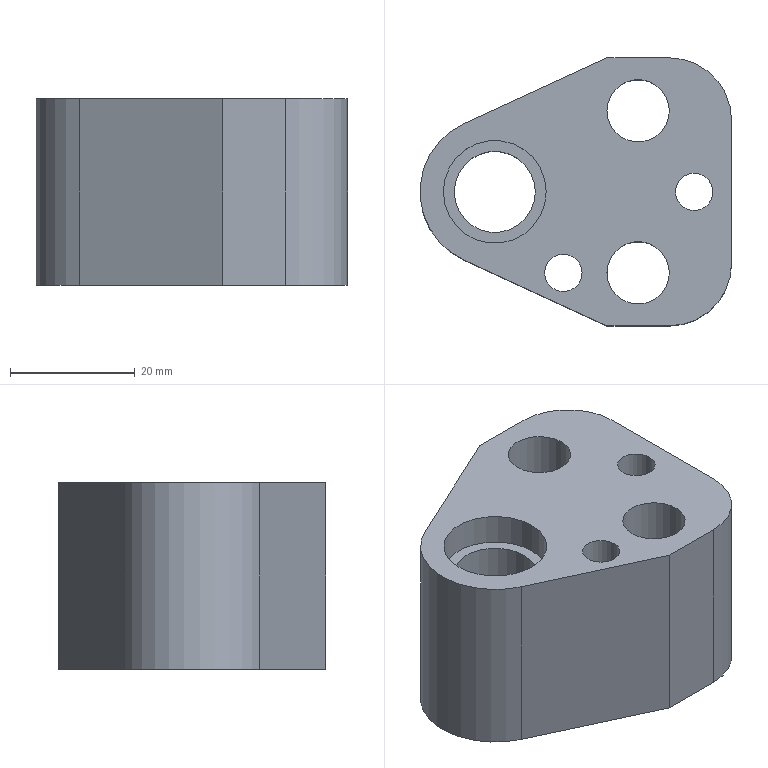Part | NX | features solid 2 | 1 solid | 25 faces | box 50 x 43 x 30 mm | volume 36983 mm3 | cylinder 13 | plane 12 | commonest cylinder face diameters 6 x2 8 x2 10 x2 14 x2 20 x2 13 x1
STEP:
#1=CARTESIAN_POINT('',(1616.,131.992,72.));
#2=VERTEX_POINT('',#1);
#3=CARTESIAN_POINT('',(1620.,131.992,72.));
#4=DIRECTION('',(0.,0.,-1.));
#5=DIRECTION('',(-1.,0.,0.));
#6=AXIS2_PLACEMENT_3D('',#3,#4,#5);
#7=CIRCLE('',#6,4.);
#8=EDGE_CURVE('',#2,#2,#7,.F.);
#9=ORIENTED_EDGE('',*,*,#8,.T.);
#10=EDGE_LOOP('',(#9));
#11=FACE_BOUND('',#10,.T.);
#12=CARTESIAN_POINT('',(1618.,118.992,72.));
#13=VERTEX_POINT('',#12);
#14=CARTESIAN_POINT('',(1611.,118.992,72.));
#15=DIRECTION('',(0.,0.,1.));
#16=DIRECTION('',(1.,0.,0.));
#17=AXIS2_PLACEMENT_3D('',#14,#15,#16);
#18=CIRCLE('',#17,7.);
#19=EDGE_CURVE('',#13,#13,#18,.T.);
#20=ORIENTED_EDGE('',*,*,#19,.T.);
#21=EDGE_LOOP('',(#20));
#22=FACE_BOUND('',#21,.T.);
#23=CARTESIAN_POINT('',(1618.,144.992,72.));
#24=VERTEX_POINT('',#23);
#25=CARTESIAN_POINT('',(1611.,144.992,72.));
#26=DIRECTION('',(0.,0.,1.));
#27=DIRECTION('',(1.,0.,0.));
#28=AXIS2_PLACEMENT_3D('',#25,#26,#27);
#29=CIRCLE('',#28,7.);
#30=EDGE_CURVE('',#24,#24,#29,.T.);
#31=ORIENTED_EDGE('',*,*,#30,.T.);
#32=EDGE_LOOP('',(#31));
#33=FACE_BOUND('',#32,.T.);
#34=CARTESIAN_POINT('',(1581.5,131.992,72.));
#35=VERTEX_POINT('',#34);
#36=CARTESIAN_POINT('',(1588.,131.992,72.));
#37=DIRECTION('',(0.,0.,-1.));
#38=DIRECTION('',(-1.,0.,0.));
#39=AXIS2_PLACEMENT_3D('',#36,#37,#38);
#40=CIRCLE('',#39,6.5);
#41=EDGE_CURVE('',#35,#35,#40,.T.);
#42=ORIENTED_EDGE('',*,*,#41,.F.);
#43=EDGE_LOOP('',(#42));
#44=FACE_BOUND('',#43,.T.);
#45=CARTESIAN_POINT('',(1582.981,142.892,72.));
#46=VERTEX_POINT('',#45);
#47=CARTESIAN_POINT('',(1606.,153.492,72.));
#48=VERTEX_POINT('',#47);
#49=CARTESIAN_POINT('',(1582.981,142.892,72.));
#50=DIRECTION('',(0.9083,0.4183,0.));
#51=VECTOR('',#50,1000.);
#52=LINE('',#49,#51);
#53=EDGE_CURVE('',#46,#48,#52,.T.);
#54=ORIENTED_EDGE('',*,*,#53,.T.);
#55=CARTESIAN_POINT('',(1616.,153.492,72.));
#56=VERTEX_POINT('',#55);
#57=CARTESIAN_POINT('',(1606.,153.492,72.));
#58=DIRECTION('',(1.,0.,0.));
#59=VECTOR('',#58,1000.);
#60=LINE('',#57,#59);
#61=EDGE_CURVE('',#48,#56,#60,.T.);
#62=ORIENTED_EDGE('',*,*,#61,.T.);
#63=CARTESIAN_POINT('',(1626.,143.492,72.));
#64=VERTEX_POINT('',#63);
#65=CARTESIAN_POINT('',(1616.,143.492,72.));
#66=DIRECTION('',(0.,0.,1.));
#67=DIRECTION('',(1.,0.,0.));
#68=AXIS2_PLACEMENT_3D('',#65,#66,#67);
#69=CIRCLE('',#68,10.);
#70=EDGE_CURVE('',#64,#56,#69,.T.);
#71=ORIENTED_EDGE('',*,*,#70,.F.);
#72=CARTESIAN_POINT('',(1626.,120.492,72.));
#73=VERTEX_POINT('',#72);
#74=CARTESIAN_POINT('',(1626.,143.492,72.));
#75=DIRECTION('',(0.,-1.,0.));
#76=VECTOR('',#75,1000.);
#77=LINE('',#74,#76);
#78=EDGE_CURVE('',#64,#73,#77,.T.);
#79=ORIENTED_EDGE('',*,*,#78,.T.);
#80=CARTESIAN_POINT('',(1616.,110.492,72.));
#81=VERTEX_POINT('',#80);
#82=CARTESIAN_POINT('',(1616.,120.492,72.));
#83=DIRECTION('',(0.,0.,1.));
#84=DIRECTION('',(1.,0.,0.));
#85=AXIS2_PLACEMENT_3D('',#82,#83,#84);
#86=CIRCLE('',#85,10.);
#87=EDGE_CURVE('',#81,#73,#86,.T.);
#88=ORIENTED_EDGE('',*,*,#87,.F.);
#89=CARTESIAN_POINT('',(1606.,110.492,72.));
#90=VERTEX_POINT('',#89);
#91=CARTESIAN_POINT('',(1606.,110.492,72.));
#92=DIRECTION('',(1.,0.,0.));
#93=VECTOR('',#92,1000.);
#94=LINE('',#91,#93);
#95=EDGE_CURVE('',#90,#81,#94,.T.);
#96=ORIENTED_EDGE('',*,*,#95,.F.);
#97=CARTESIAN_POINT('',(1582.981,121.093,72.));
#98=VERTEX_POINT('',#97);
#99=CARTESIAN_POINT('',(1582.981,121.093,72.));
#100=DIRECTION('',(0.9083,-0.4183,0.));
#101=VECTOR('',#100,1000.);
#102=LINE('',#99,#101);
#103=EDGE_CURVE('',#98,#90,#102,.T.);
#104=ORIENTED_EDGE('',*,*,#103,.F.);
#105=CARTESIAN_POINT('',(1588.,131.992,72.));
#106=DIRECTION('',(0.,0.,1.));
#107=DIRECTION('',(1.,0.,0.));
#108=AXIS2_PLACEMENT_3D('',#105,#106,#107);
#109=CIRCLE('',#108,12.);
#110=EDGE_CURVE('',#46,#98,#109,.T.);
#111=ORIENTED_EDGE('',*,*,#110,.F.);
#112=EDGE_LOOP('',(#54,#62,#71,#79,#88,#96,#104,#111));
#113=FACE_BOUND('',#112,.T.);
#114=CARTESIAN_POINT('',(1595.,118.992,72.));
#115=VERTEX_POINT('',#114);
#116=CARTESIAN_POINT('',(1599.,118.992,72.));
#117=DIRECTION('',(0.,0.,-1.));
#118=DIRECTION('',(-1.,0.,0.));
#119=AXIS2_PLACEMENT_3D('',#116,#117,#118);
#120=CIRCLE('',#119,4.);
#121=EDGE_CURVE('',#115,#115,#120,.F.);
#122=ORIENTED_EDGE('',*,*,#121,.T.);
#123=EDGE_LOOP('',(#122));
#124=FACE_BOUND('',#123,.T.);
#125=CARTESIAN_POINT('',(1616.,143.492,72.));
#126=DIRECTION('',(0.,0.,-1.));
#127=DIRECTION('',(1.,0.,0.));
#128=AXIS2_PLACEMENT_3D('',#125,#126,#127);
#129=PLANE('',#128);
#130=ADVANCED_FACE('',(#11,#22,#33,#44,#113,#124),#129,.T.);
#131=CARTESIAN_POINT('',(1623.,131.992,102.));
#132=VERTEX_POINT('',#131);
#133=CARTESIAN_POINT('',(1620.,131.992,102.));
#134=DIRECTION('',(0.,0.,1.));
#135=DIRECTION('',(1.,0.,0.));
#136=AXIS2_PLACEMENT_3D('',#133,#134,#135);
#137=CIRCLE('',#136,3.);
#138=EDGE_CURVE('',#132,#132,#137,.T.);
#139=ORIENTED_EDGE('',*,*,#138,.T.);
#140=EDGE_LOOP('',(#139));
#141=FACE_BOUND('',#140,.T.);
#142=CARTESIAN_POINT('',(1623.,131.992,92.));
#143=VERTEX_POINT('',#142);
#144=CARTESIAN_POINT('',(1620.,131.992,92.));
#145=DIRECTION('',(0.,0.,1.));
#146=DIRECTION('',(1.,0.,0.));
#147=AXIS2_PLACEMENT_3D('',#144,#145,#146);
#148=CIRCLE('',#147,3.);
#149=EDGE_CURVE('',#143,#143,#148,.T.);
#150=ORIENTED_EDGE('',*,*,#149,.F.);
#151=EDGE_LOOP('',(#150));
#152=FACE_BOUND('',#151,.T.);
#153=CARTESIAN_POINT('',(1620.,131.992,72.));
#154=DIRECTION('',(0.,0.,1.));
#155=DIRECTION('',(-1.,0.,0.));
#156=AXIS2_PLACEMENT_3D('',#153,#154,#155);
#157=CYLINDRICAL_SURFACE('',#156,3.);
#158=ADVANCED_FACE('',(#141,#152),#157,.F.);
#159=CARTESIAN_POINT('',(1616.,118.992,102.));
#160=VERTEX_POINT('',#159);
#161=CARTESIAN_POINT('',(1611.,118.992,102.));
#162=DIRECTION('',(0.,0.,1.));
#163=DIRECTION('',(1.,0.,0.));
#164=AXIS2_PLACEMENT_3D('',#161,#162,#163);
#165=CIRCLE('',#164,5.);
#166=EDGE_CURVE('',#160,#160,#165,.T.);
#167=ORIENTED_EDGE('',*,*,#166,.T.);
#168=EDGE_LOOP('',(#167));
#169=FACE_BOUND('',#168,.T.);
#170=CARTESIAN_POINT('',(1616.,118.992,82.));
#171=VERTEX_POINT('',#170);
#172=CARTESIAN_POINT('',(1611.,118.992,82.));
#173=DIRECTION('',(0.,0.,1.));
#174=DIRECTION('',(1.,0.,0.));
#175=AXIS2_PLACEMENT_3D('',#172,#173,#174);
#176=CIRCLE('',#175,5.);
#177=EDGE_CURVE('',#171,#171,#176,.T.);
#178=ORIENTED_EDGE('',*,*,#177,.F.);
#179=EDGE_LOOP('',(#178));
#180=FACE_BOUND('',#179,.T.);
#181=CARTESIAN_POINT('',(1611.,118.992,72.));
#182=DIRECTION('',(0.,0.,1.));
#183=DIRECTION('',(-1.,0.,0.));
#184=AXIS2_PLACEMENT_3D('',#181,#182,#183);
#185=CYLINDRICAL_SURFACE('',#184,5.);
#186=ADVANCED_FACE('',(#169,#180),#185,.F.);
#187=CARTESIAN_POINT('',(1616.,144.992,102.));
#188=VERTEX_POINT('',#187);
#189=CARTESIAN_POINT('',(1611.,144.992,102.));
#190=DIRECTION('',(0.,0.,1.));
#191=DIRECTION('',(1.,0.,0.));
#192=AXIS2_PLACEMENT_3D('',#189,#190,#191);
#193=CIRCLE('',#192,5.);
#194=EDGE_CURVE('',#188,#188,#193,.T.);
#195=ORIENTED_EDGE('',*,*,#194,.T.);
#196=EDGE_LOOP('',(#195));
#197=FACE_BOUND('',#196,.T.);
#198=CARTESIAN_POINT('',(1616.,144.992,82.));
#199=VERTEX_POINT('',#198);
#200=CARTESIAN_POINT('',(1611.,144.992,82.));
#201=DIRECTION('',(0.,0.,1.));
#202=DIRECTION('',(1.,0.,0.));
#203=AXIS2_PLACEMENT_3D('',#200,#201,#202);
#204=CIRCLE('',#203,5.);
#205=EDGE_CURVE('',#199,#199,#204,.T.);
#206=ORIENTED_EDGE('',*,*,#205,.F.);
#207=EDGE_LOOP('',(#206));
#208=FACE_BOUND('',#207,.T.);
#209=CARTESIAN_POINT('',(1611.,144.992,72.));
#210=DIRECTION('',(0.,0.,1.));
#211=DIRECTION('',(-1.,0.,0.));
#212=AXIS2_PLACEMENT_3D('',#209,#210,#211);
#213=CYLINDRICAL_SURFACE('',#212,5.);
#214=ADVANCED_FACE('',(#197,#208),#213,.F.);
#215=CARTESIAN_POINT('',(1602.,118.992,102.));
#216=VERTEX_POINT('',#215);
#217=CARTESIAN_POINT('',(1599.,118.992,102.));
#218=DIRECTION('',(0.,0.,1.));
#219=DIRECTION('',(1.,0.,0.));
#220=AXIS2_PLACEMENT_3D('',#217,#218,#219);
#221=CIRCLE('',#220,3.);
#222=EDGE_CURVE('',#216,#216,#221,.T.);
#223=ORIENTED_EDGE('',*,*,#222,.F.);
#224=EDGE_LOOP('',(#223));
#225=FACE_BOUND('',#224,.T.);
#226=ORIENTED_EDGE('',*,*,#166,.F.);
#227=EDGE_LOOP('',(#226));
#228=FACE_BOUND('',#227,.T.);
#229=CARTESIAN_POINT('',(1582.981,142.892,102.));
#230=VERTEX_POINT('',#229);
#231=CARTESIAN_POINT('',(1606.,153.492,102.));
#232=VERTEX_POINT('',#231);
#233=CARTESIAN_POINT('',(1582.981,142.892,102.));
#234=DIRECTION('',(0.9083,0.4183,0.));
#235=VECTOR('',#234,1000.);
#236=LINE('',#233,#235);
#237=EDGE_CURVE('',#230,#232,#236,.T.);
#238=ORIENTED_EDGE('',*,*,#237,.F.);
#239=CARTESIAN_POINT('',(1582.981,121.093,102.));
#240=VERTEX_POINT('',#239);
#241=CARTESIAN_POINT('',(1588.,131.992,102.));
#242=DIRECTION('',(0.,0.,1.));
#243=DIRECTION('',(1.,0.,0.));
#244=AXIS2_PLACEMENT_3D('',#241,#242,#243);
#245=CIRCLE('',#244,12.);
#246=EDGE_CURVE('',#230,#240,#245,.T.);
#247=ORIENTED_EDGE('',*,*,#246,.T.);
#248=CARTESIAN_POINT('',(1606.,110.492,102.));
#249=VERTEX_POINT('',#248);
#250=CARTESIAN_POINT('',(1582.981,121.093,102.));
#251=DIRECTION('',(0.9083,-0.4183,0.));
#252=VECTOR('',#251,1000.);
#253=LINE('',#250,#252);
#254=EDGE_CURVE('',#240,#249,#253,.T.);
#255=ORIENTED_EDGE('',*,*,#254,.T.);
#256=CARTESIAN_POINT('',(1616.,110.492,102.));
#257=VERTEX_POINT('',#256);
#258=CARTESIAN_POINT('',(1606.,110.492,102.));
#259=DIRECTION('',(1.,0.,0.));
#260=VECTOR('',#259,1000.);
#261=LINE('',#258,#260);
#262=EDGE_CURVE('',#249,#257,#261,.T.);
#263=ORIENTED_EDGE('',*,*,#262,.T.);
#264=CARTESIAN_POINT('',(1626.,120.492,102.));
#265=VERTEX_POINT('',#264);
#266=CARTESIAN_POINT('',(1616.,120.492,102.));
#267=DIRECTION('',(0.,0.,1.));
#268=DIRECTION('',(1.,0.,0.));
#269=AXIS2_PLACEMENT_3D('',#266,#267,#268);
#270=CIRCLE('',#269,10.);
#271=EDGE_CURVE('',#257,#265,#270,.T.);
#272=ORIENTED_EDGE('',*,*,#271,.T.);
#273=CARTESIAN_POINT('',(1626.,143.492,102.));
#274=VERTEX_POINT('',#273);
#275=CARTESIAN_POINT('',(1626.,143.492,102.));
#276=DIRECTION('',(0.,-1.,0.));
#277=VECTOR('',#276,1000.);
#278=LINE('',#275,#277);
#279=EDGE_CURVE('',#274,#265,#278,.T.);
#280=ORIENTED_EDGE('',*,*,#279,.F.);
#281=CARTESIAN_POINT('',(1616.,153.492,102.));
#282=VERTEX_POINT('',#281);
#283=CARTESIAN_POINT('',(1616.,143.492,102.));
#284=DIRECTION('',(0.,0.,1.));
#285=DIRECTION('',(1.,0.,0.));
#286=AXIS2_PLACEMENT_3D('',#283,#284,#285);
#287=CIRCLE('',#286,10.);
#288=EDGE_CURVE('',#274,#282,#287,.T.);
#289=ORIENTED_EDGE('',*,*,#288,.T.);
#290=CARTESIAN_POINT('',(1606.,153.492,102.));
#291=DIRECTION('',(1.,0.,0.));
#292=VECTOR('',#291,1000.);
#293=LINE('',#290,#292);
#294=EDGE_CURVE('',#232,#282,#293,.T.);
#295=ORIENTED_EDGE('',*,*,#294,.F.);
#296=EDGE_LOOP('',(#238,#247,#255,#263,#272,#280,#289,#295));
#297=FACE_BOUND('',#296,.T.);
#298=CARTESIAN_POINT('',(1596.25,131.992,102.));
#299=VERTEX_POINT('',#298);
#300=CARTESIAN_POINT('',(1588.,131.992,102.));
#301=DIRECTION('',(0.,0.,1.));
#302=DIRECTION('',(1.,0.,0.));
#303=AXIS2_PLACEMENT_3D('',#300,#301,#302);
#304=CIRCLE('',#303,8.25);
#305=EDGE_CURVE('',#299,#299,#304,.T.);
#306=ORIENTED_EDGE('',*,*,#305,.F.);
#307=EDGE_LOOP('',(#306));
#308=FACE_BOUND('',#307,.T.);
#309=ORIENTED_EDGE('',*,*,#194,.F.);
#310=EDGE_LOOP('',(#309));
#311=FACE_BOUND('',#310,.T.);
#312=ORIENTED_EDGE('',*,*,#138,.F.);
#313=EDGE_LOOP('',(#312));
#314=FACE_BOUND('',#313,.T.);
#315=CARTESIAN_POINT('',(1616.,143.492,102.));
#316=DIRECTION('',(0.,0.,-1.));
#317=DIRECTION('',(1.,0.,0.));
#318=AXIS2_PLACEMENT_3D('',#315,#316,#317);
#319=PLANE('',#318);
#320=ADVANCED_FACE('',(#225,#228,#297,#308,#311,#314),#319,.F.);
#321=ORIENTED_EDGE('',*,*,#237,.T.);
#322=CARTESIAN_POINT('',(1606.,153.492,72.));
#323=DIRECTION('',(0.,0.,1.));
#324=VECTOR('',#323,1000.);
#325=LINE('',#322,#324);
#326=EDGE_CURVE('',#48,#232,#325,.T.);
#327=ORIENTED_EDGE('',*,*,#326,.F.);
#328=ORIENTED_EDGE('',*,*,#53,.F.);
#329=CARTESIAN_POINT('',(1582.981,142.892,72.));
#330=DIRECTION('',(0.,0.,1.));
#331=VECTOR('',#330,1000.);
#332=LINE('',#329,#331);
#333=EDGE_CURVE('',#46,#230,#332,.T.);
#334=ORIENTED_EDGE('',*,*,#333,.T.);
#335=EDGE_LOOP('',(#321,#327,#328,#334));
#336=FACE_BOUND('',#335,.T.);
#337=CARTESIAN_POINT('',(1582.981,142.892,72.));
#338=DIRECTION('',(-0.4183,0.9083,0.));
#339=DIRECTION('',(0.9083,0.4183,0.));
#340=AXIS2_PLACEMENT_3D('',#337,#338,#339);
#341=PLANE('',#340);
#342=ADVANCED_FACE('',(#336),#341,.T.);
#343=ORIENTED_EDGE('',*,*,#294,.T.);
#344=CARTESIAN_POINT('',(1616.,153.492,72.));
#345=DIRECTION('',(0.,0.,1.));
#346=VECTOR('',#345,1000.);
#347=LINE('',#344,#346);
#348=EDGE_CURVE('',#56,#282,#347,.T.);
#349=ORIENTED_EDGE('',*,*,#348,.F.);
#350=ORIENTED_EDGE('',*,*,#61,.F.);
#351=ORIENTED_EDGE('',*,*,#326,.T.);
#352=EDGE_LOOP('',(#343,#349,#350,#351));
#353=FACE_BOUND('',#352,.T.);
#354=CARTESIAN_POINT('',(1606.,153.492,72.));
#355=DIRECTION('',(0.,1.,0.));
#356=DIRECTION('',(1.,0.,0.));
#357=AXIS2_PLACEMENT_3D('',#354,#355,#356);
#358=PLANE('',#357);
#359=ADVANCED_FACE('',(#353),#358,.T.);
#360=ORIENTED_EDGE('',*,*,#288,.F.);
#361=CARTESIAN_POINT('',(1626.,143.492,72.));
#362=DIRECTION('',(0.,0.,1.));
#363=VECTOR('',#362,1000.);
#364=LINE('',#361,#363);
#365=EDGE_CURVE('',#64,#274,#364,.T.);
#366=ORIENTED_EDGE('',*,*,#365,.F.);
#367=ORIENTED_EDGE('',*,*,#70,.T.);
#368=ORIENTED_EDGE('',*,*,#348,.T.);
#369=EDGE_LOOP('',(#360,#366,#367,#368));
#370=FACE_BOUND('',#369,.T.);
#371=CARTESIAN_POINT('',(1616.,143.492,72.));
#372=DIRECTION('',(0.,0.,1.));
#373=DIRECTION('',(-1.,0.,0.));
#374=AXIS2_PLACEMENT_3D('',#371,#372,#373);
#375=CYLINDRICAL_SURFACE('',#374,10.);
#376=ADVANCED_FACE('',(#370),#375,.T.);
#377=ORIENTED_EDGE('',*,*,#279,.T.);
#378=CARTESIAN_POINT('',(1626.,120.492,72.));
#379=DIRECTION('',(0.,0.,1.));
#380=VECTOR('',#379,1000.);
#381=LINE('',#378,#380);
#382=EDGE_CURVE('',#73,#265,#381,.T.);
#383=ORIENTED_EDGE('',*,*,#382,.F.);
#384=ORIENTED_EDGE('',*,*,#78,.F.);
#385=ORIENTED_EDGE('',*,*,#365,.T.);
#386=EDGE_LOOP('',(#377,#383,#384,#385));
#387=FACE_BOUND('',#386,.T.);
#388=CARTESIAN_POINT('',(1626.,143.492,72.));
#389=DIRECTION('',(1.,0.,0.));
#390=DIRECTION('',(0.,-1.,0.));
#391=AXIS2_PLACEMENT_3D('',#388,#389,#390);
#392=PLANE('',#391);
#393=ADVANCED_FACE('',(#387),#392,.T.);
#394=ORIENTED_EDGE('',*,*,#271,.F.);
#395=CARTESIAN_POINT('',(1616.,110.492,72.));
#396=DIRECTION('',(0.,0.,1.));
#397=VECTOR('',#396,1000.);
#398=LINE('',#395,#397);
#399=EDGE_CURVE('',#81,#257,#398,.T.);
#400=ORIENTED_EDGE('',*,*,#399,.F.);
#401=ORIENTED_EDGE('',*,*,#87,.T.);
#402=ORIENTED_EDGE('',*,*,#382,.T.);
#403=EDGE_LOOP('',(#394,#400,#401,#402));
#404=FACE_BOUND('',#403,.T.);
#405=CARTESIAN_POINT('',(1616.,120.492,72.));
#406=DIRECTION('',(0.,0.,1.));
#407=DIRECTION('',(-1.,0.,0.));
#408=AXIS2_PLACEMENT_3D('',#405,#406,#407);
#409=CYLINDRICAL_SURFACE('',#408,10.);
#410=ADVANCED_FACE('',(#404),#409,.T.);
#411=ORIENTED_EDGE('',*,*,#262,.F.);
#412=CARTESIAN_POINT('',(1606.,110.492,72.));
#413=DIRECTION('',(0.,0.,1.));
#414=VECTOR('',#413,1000.);
#415=LINE('',#412,#414);
#416=EDGE_CURVE('',#90,#249,#415,.T.);
#417=ORIENTED_EDGE('',*,*,#416,.F.);
#418=ORIENTED_EDGE('',*,*,#95,.T.);
#419=ORIENTED_EDGE('',*,*,#399,.T.);
#420=EDGE_LOOP('',(#411,#417,#418,#419));
#421=FACE_BOUND('',#420,.T.);
#422=CARTESIAN_POINT('',(1606.,110.492,72.));
#423=DIRECTION('',(0.,1.,0.));
#424=DIRECTION('',(1.,0.,0.));
#425=AXIS2_PLACEMENT_3D('',#422,#423,#424);
#426=PLANE('',#425);
#427=ADVANCED_FACE('',(#421),#426,.F.);
#428=ORIENTED_EDGE('',*,*,#254,.F.);
#429=CARTESIAN_POINT('',(1582.981,121.093,72.));
#430=DIRECTION('',(0.,0.,1.));
#431=VECTOR('',#430,1000.);
#432=LINE('',#429,#431);
#433=EDGE_CURVE('',#98,#240,#432,.T.);
#434=ORIENTED_EDGE('',*,*,#433,.F.);
#435=ORIENTED_EDGE('',*,*,#103,.T.);
#436=ORIENTED_EDGE('',*,*,#416,.T.);
#437=EDGE_LOOP('',(#428,#434,#435,#436));
#438=FACE_BOUND('',#437,.T.);
#439=CARTESIAN_POINT('',(1582.981,121.093,72.));
#440=DIRECTION('',(0.4183,0.9083,0.));
#441=DIRECTION('',(0.9083,-0.4183,0.));
#442=AXIS2_PLACEMENT_3D('',#439,#440,#441);
#443=PLANE('',#442);
#444=ADVANCED_FACE('',(#438),#443,.F.);
#445=ORIENTED_EDGE('',*,*,#246,.F.);
#446=ORIENTED_EDGE('',*,*,#333,.F.);
#447=ORIENTED_EDGE('',*,*,#110,.T.);
#448=ORIENTED_EDGE('',*,*,#433,.T.);
#449=EDGE_LOOP('',(#445,#446,#447,#448));
#450=FACE_BOUND('',#449,.T.);
#451=CARTESIAN_POINT('',(1588.,131.992,72.));
#452=DIRECTION('',(0.,0.,1.));
#453=DIRECTION('',(-1.,0.,0.));
#454=AXIS2_PLACEMENT_3D('',#451,#452,#453);
#455=CYLINDRICAL_SURFACE('',#454,12.);
#456=ADVANCED_FACE('',(#450),#455,.T.);
#457=CARTESIAN_POINT('',(1594.5,131.992,97.));
#458=VERTEX_POINT('',#457);
#459=CARTESIAN_POINT('',(1588.,131.992,97.));
#460=DIRECTION('',(0.,0.,1.));
#461=DIRECTION('',(1.,0.,0.));
#462=AXIS2_PLACEMENT_3D('',#459,#460,#461);
#463=CIRCLE('',#462,6.5);
#464=EDGE_CURVE('',#458,#458,#463,.F.);
#465=ORIENTED_EDGE('',*,*,#464,.F.);
#466=EDGE_LOOP('',(#465));
#467=FACE_BOUND('',#466,.T.);
#468=ORIENTED_EDGE('',*,*,#41,.T.);
#469=EDGE_LOOP('',(#468));
#470=FACE_BOUND('',#469,.T.);
#471=CARTESIAN_POINT('',(1588.,131.992,72.));
#472=DIRECTION('',(0.,0.,1.));
#473=DIRECTION('',(-1.,0.,0.));
#474=AXIS2_PLACEMENT_3D('',#471,#472,#473);
#475=CYLINDRICAL_SURFACE('',#474,6.5);
#476=ADVANCED_FACE('',(#467,#470),#475,.F.);
#477=CARTESIAN_POINT('',(1596.25,131.992,97.));
#478=VERTEX_POINT('',#477);
#479=CARTESIAN_POINT('',(1588.,131.992,97.));
#480=DIRECTION('',(0.,0.,1.));
#481=DIRECTION('',(1.,0.,0.));
#482=AXIS2_PLACEMENT_3D('',#479,#480,#481);
#483=CIRCLE('',#482,8.25);
#484=EDGE_CURVE('',#478,#478,#483,.T.);
#485=ORIENTED_EDGE('',*,*,#484,.T.);
#486=EDGE_LOOP('',(#485));
#487=FACE_BOUND('',#486,.T.);
#488=ORIENTED_EDGE('',*,*,#464,.T.);
#489=EDGE_LOOP('',(#488));
#490=FACE_BOUND('',#489,.T.);
#491=CARTESIAN_POINT('',(1588.,131.992,97.));
#492=DIRECTION('',(0.,0.,-1.));
#493=DIRECTION('',(1.,0.,0.));
#494=AXIS2_PLACEMENT_3D('',#491,#492,#493);
#495=PLANE('',#494);
#496=ADVANCED_FACE('',(#487,#490),#495,.F.);
#497=ORIENTED_EDGE('',*,*,#484,.F.);
#498=EDGE_LOOP('',(#497));
#499=FACE_BOUND('',#498,.T.);
#500=ORIENTED_EDGE('',*,*,#305,.T.);
#501=EDGE_LOOP('',(#500));
#502=FACE_BOUND('',#501,.T.);
#503=CARTESIAN_POINT('',(1588.,131.992,97.));
#504=DIRECTION('',(0.,0.,1.));
#505=DIRECTION('',(-1.,0.,0.));
#506=AXIS2_PLACEMENT_3D('',#503,#504,#505);
#507=CYLINDRICAL_SURFACE('',#506,8.25);
#508=ADVANCED_FACE('',(#499,#502),#507,.F.);
#509=CARTESIAN_POINT('',(1602.,118.992,92.));
#510=VERTEX_POINT('',#509);
#511=CARTESIAN_POINT('',(1599.,118.992,92.));
#512=DIRECTION('',(0.,0.,1.));
#513=DIRECTION('',(1.,0.,0.));
#514=AXIS2_PLACEMENT_3D('',#511,#512,#513);
#515=CIRCLE('',#514,3.);
#516=EDGE_CURVE('',#510,#510,#515,.T.);
#517=ORIENTED_EDGE('',*,*,#516,.F.);
#518=EDGE_LOOP('',(#517));
#519=FACE_BOUND('',#518,.T.);
#520=ORIENTED_EDGE('',*,*,#222,.T.);
#521=EDGE_LOOP('',(#520));
#522=FACE_BOUND('',#521,.T.);
#523=CARTESIAN_POINT('',(1599.,118.992,72.));
#524=DIRECTION('',(0.,0.,1.));
#525=DIRECTION('',(-1.,0.,0.));
#526=AXIS2_PLACEMENT_3D('',#523,#524,#525);
#527=CYLINDRICAL_SURFACE('',#526,3.);
#528=ADVANCED_FACE('',(#519,#522),#527,.F.);
#529=CARTESIAN_POINT('',(1618.,144.992,82.));
#530=VERTEX_POINT('',#529);
#531=CARTESIAN_POINT('',(1611.,144.992,82.));
#532=DIRECTION('',(0.,0.,1.));
#533=DIRECTION('',(1.,0.,0.));
#534=AXIS2_PLACEMENT_3D('',#531,#532,#533);
#535=CIRCLE('',#534,7.);
#536=EDGE_CURVE('',#530,#530,#535,.T.);
#537=ORIENTED_EDGE('',*,*,#536,.T.);
#538=EDGE_LOOP('',(#537));
#539=FACE_BOUND('',#538,.T.);
#540=ORIENTED_EDGE('',*,*,#30,.F.);
#541=EDGE_LOOP('',(#540));
#542=FACE_BOUND('',#541,.T.);
#543=CARTESIAN_POINT('',(1611.,144.992,82.));
#544=DIRECTION('',(0.,0.,-1.));
#545=DIRECTION('',(1.,0.,0.));
#546=AXIS2_PLACEMENT_3D('',#543,#544,#545);
#547=CYLINDRICAL_SURFACE('',#546,7.);
#548=ADVANCED_FACE('',(#539,#542),#547,.F.);
#549=ORIENTED_EDGE('',*,*,#205,.T.);
#550=EDGE_LOOP('',(#549));
#551=FACE_BOUND('',#550,.T.);
#552=ORIENTED_EDGE('',*,*,#536,.F.);
#553=EDGE_LOOP('',(#552));
#554=FACE_BOUND('',#553,.T.);
#555=CARTESIAN_POINT('',(1611.,144.992,82.));
#556=DIRECTION('',(0.,0.,-1.));
#557=DIRECTION('',(1.,0.,0.));
#558=AXIS2_PLACEMENT_3D('',#555,#556,#557);
#559=PLANE('',#558);
#560=ADVANCED_FACE('',(#551,#554),#559,.T.);
#561=CARTESIAN_POINT('',(1618.,118.992,82.));
#562=VERTEX_POINT('',#561);
#563=CARTESIAN_POINT('',(1611.,118.992,82.));
#564=DIRECTION('',(0.,0.,1.));
#565=DIRECTION('',(1.,0.,0.));
#566=AXIS2_PLACEMENT_3D('',#563,#564,#565);
#567=CIRCLE('',#566,7.);
#568=EDGE_CURVE('',#562,#562,#567,.T.);
#569=ORIENTED_EDGE('',*,*,#568,.T.);
#570=EDGE_LOOP('',(#569));
#571=FACE_BOUND('',#570,.T.);
#572=ORIENTED_EDGE('',*,*,#19,.F.);
#573=EDGE_LOOP('',(#572));
#574=FACE_BOUND('',#573,.T.);
#575=CARTESIAN_POINT('',(1611.,118.992,82.));
#576=DIRECTION('',(0.,0.,-1.));
#577=DIRECTION('',(1.,0.,0.));
#578=AXIS2_PLACEMENT_3D('',#575,#576,#577);
#579=CYLINDRICAL_SURFACE('',#578,7.);
#580=ADVANCED_FACE('',(#571,#574),#579,.F.);
#581=ORIENTED_EDGE('',*,*,#177,.T.);
#582=EDGE_LOOP('',(#581));
#583=FACE_BOUND('',#582,.T.);
#584=ORIENTED_EDGE('',*,*,#568,.F.);
#585=EDGE_LOOP('',(#584));
#586=FACE_BOUND('',#585,.T.);
#587=CARTESIAN_POINT('',(1611.,118.992,82.));
#588=DIRECTION('',(0.,0.,-1.));
#589=DIRECTION('',(1.,0.,0.));
#590=AXIS2_PLACEMENT_3D('',#587,#588,#589);
#591=PLANE('',#590);
#592=ADVANCED_FACE('',(#583,#586),#591,.T.);
#593=ORIENTED_EDGE('',*,*,#149,.T.);
#594=EDGE_LOOP('',(#593));
#595=FACE_BOUND('',#594,.T.);
#596=CARTESIAN_POINT('',(1616.,131.992,92.));
#597=VERTEX_POINT('',#596);
#598=CARTESIAN_POINT('',(1620.,131.992,92.));
#599=DIRECTION('',(0.,0.,-1.));
#600=DIRECTION('',(-1.,0.,0.));
#601=AXIS2_PLACEMENT_3D('',#598,#599,#600);
#602=CIRCLE('',#601,4.);
#603=EDGE_CURVE('',#597,#597,#602,.F.);
#604=ORIENTED_EDGE('',*,*,#603,.F.);
#605=EDGE_LOOP('',(#604));
#606=FACE_BOUND('',#605,.T.);
#607=CARTESIAN_POINT('',(1620.,131.992,92.));
#608=DIRECTION('',(0.,0.,1.));
#609=DIRECTION('',(-1.,0.,0.));
#610=AXIS2_PLACEMENT_3D('',#607,#608,#609);
#611=PLANE('',#610);
#612=ADVANCED_FACE('',(#595,#606),#611,.F.);
#613=ORIENTED_EDGE('',*,*,#603,.T.);
#614=EDGE_LOOP('',(#613));
#615=FACE_BOUND('',#614,.T.);
#616=ORIENTED_EDGE('',*,*,#8,.F.);
#617=EDGE_LOOP('',(#616));
#618=FACE_BOUND('',#617,.T.);
#619=CARTESIAN_POINT('',(1620.,131.992,72.));
#620=DIRECTION('',(0.,0.,1.));
#621=DIRECTION('',(-1.,0.,0.));
#622=AXIS2_PLACEMENT_3D('',#619,#620,#621);
#623=CYLINDRICAL_SURFACE('',#622,4.);
#624=ADVANCED_FACE('',(#615,#618),#623,.F.);
#625=ORIENTED_EDGE('',*,*,#516,.T.);
#626=EDGE_LOOP('',(#625));
#627=FACE_BOUND('',#626,.T.);
#628=CARTESIAN_POINT('',(1595.,118.992,92.));
#629=VERTEX_POINT('',#628);
#630=CARTESIAN_POINT('',(1599.,118.992,92.));
#631=DIRECTION('',(0.,0.,-1.));
#632=DIRECTION('',(-1.,0.,0.));
#633=AXIS2_PLACEMENT_3D('',#630,#631,#632);
#634=CIRCLE('',#633,4.);
#635=EDGE_CURVE('',#629,#629,#634,.F.);
#636=ORIENTED_EDGE('',*,*,#635,.F.);
#637=EDGE_LOOP('',(#636));
#638=FACE_BOUND('',#637,.T.);
#639=CARTESIAN_POINT('',(1599.,118.992,92.));
#640=DIRECTION('',(0.,0.,1.));
#641=DIRECTION('',(-1.,0.,0.));
#642=AXIS2_PLACEMENT_3D('',#639,#640,#641);
#643=PLANE('',#642);
#644=ADVANCED_FACE('',(#627,#638),#643,.F.);
#645=ORIENTED_EDGE('',*,*,#635,.T.);
#646=EDGE_LOOP('',(#645));
#647=FACE_BOUND('',#646,.T.);
#648=ORIENTED_EDGE('',*,*,#121,.F.);
#649=EDGE_LOOP('',(#648));
#650=FACE_BOUND('',#649,.T.);
#651=CARTESIAN_POINT('',(1599.,118.992,72.));
#652=DIRECTION('',(0.,0.,1.));
#653=DIRECTION('',(-1.,0.,0.));
#654=AXIS2_PLACEMENT_3D('',#651,#652,#653);
#655=CYLINDRICAL_SURFACE('',#654,4.);
#656=ADVANCED_FACE('',(#647,#650),#655,.F.);
#657=CLOSED_SHELL('',(#130,#158,#186,#214,#320,#342,#359,#376,#393,#410,#427,#444,#456,#476,#496,#508,#528,#548,#560,#580,#592,#612,#624,#644,#656));
#658=MANIFOLD_SOLID_BREP('',#657);
#659=(LENGTH_UNIT()NAMED_UNIT(*)SI_UNIT(.MILLI.,.METRE.));
#660=UNCERTAINTY_MEASURE_WITH_UNIT(LENGTH_MEASURE(0.00001),#659,'','');
#661=(NAMED_UNIT(*)PLANE_ANGLE_UNIT()SI_UNIT($,.RADIAN.));
#662=(NAMED_UNIT(*)SI_UNIT($,.STERADIAN.)SOLID_ANGLE_UNIT());
#663=(GEOMETRIC_REPRESENTATION_CONTEXT(3)GLOBAL_UNCERTAINTY_ASSIGNED_CONTEXT((#660))GLOBAL_UNIT_ASSIGNED_CONTEXT((#659,#661,#662))REPRESENTATION_CONTEXT('',''));
#664=ADVANCED_BREP_SHAPE_REPRESENTATION('',(#658),#663);